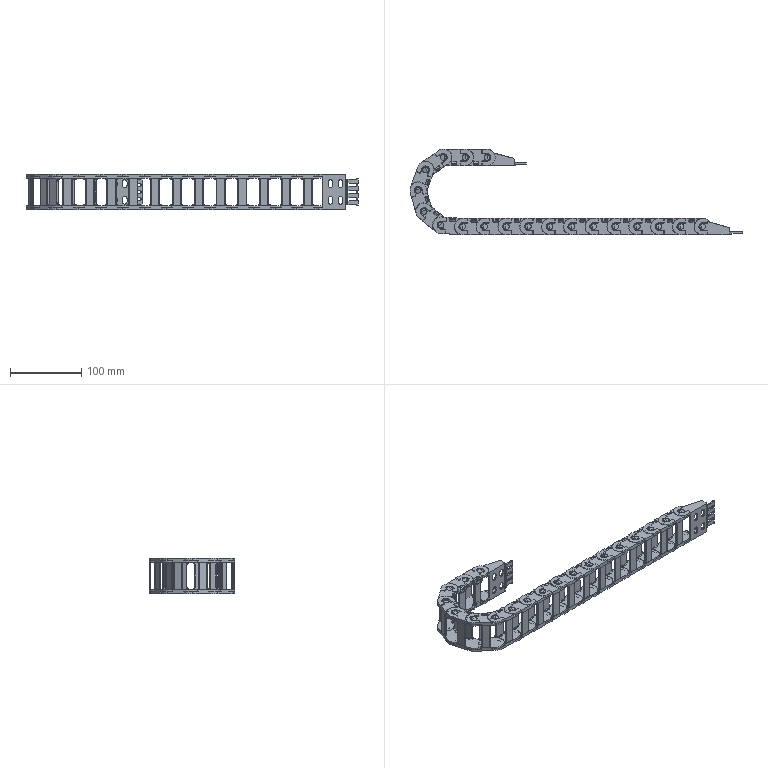Part | SolidWorks | 20 solids | 4788 faces | volume 173847 mm3 | cylinder 2268 | plane 2226 | spline 156 | cone 138 | commonest cylinder face diameters 1 x482 0.6 x270 2 x186 1.2 x117 8 x116 23 x112